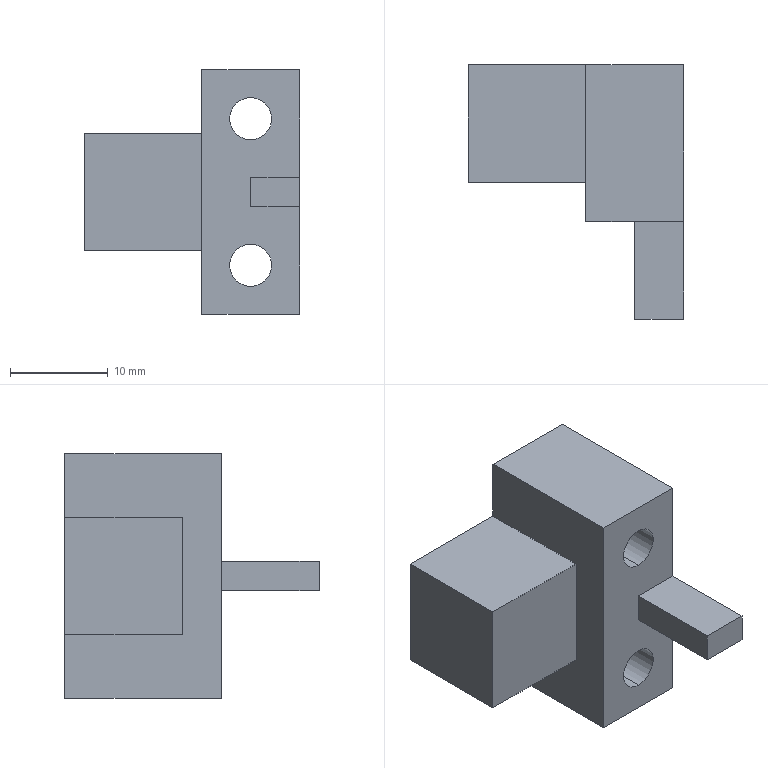Part | STEP file | Locating block | 1 solid | 24 faces | box 22 x 26 x 25 mm | volume 4984 mm3 | plane 16 | cylinder 8 | commonest cylinder face diameters 4.3 x4 8 x4